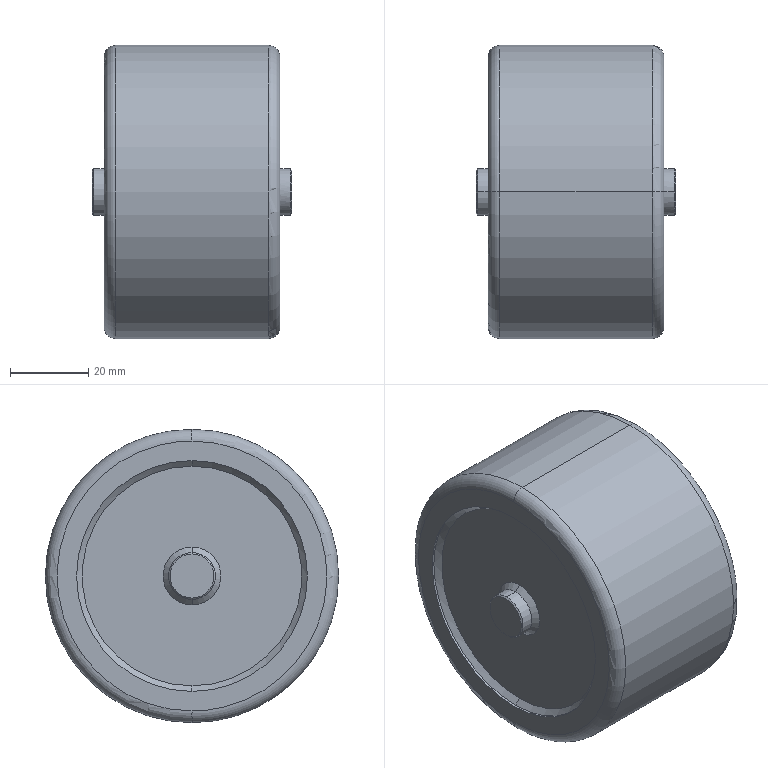Part | SolidWorks | features BaseBody 1 | 1 solid | 32 faces | box 51 x 75 x 75 mm | volume 191030 mm3 | cone 12 | cylinder 10 | plane 6 | torus 4 | commonest cylinder face diameters 12 x4 59 x4 75 x2